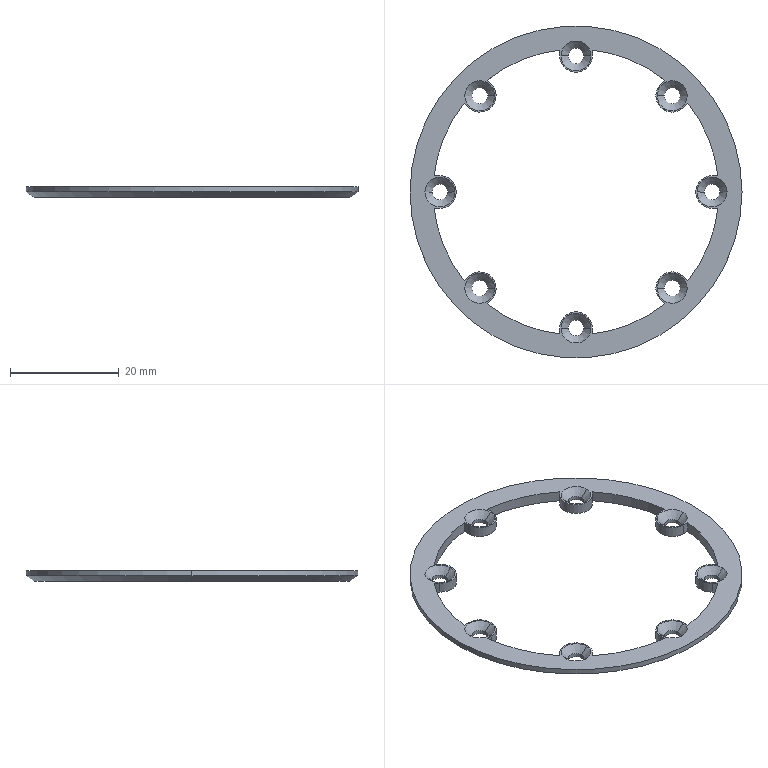Part | SolidWorks | features Chamfer 1, CirPattern 1, Extrusion 1, HoleWzd 1, ICE 1 | 1 solid | 73 faces | box 61 x 61 x 2 mm | volume 1529 mm3 | cylinder 37 | cone 18 | plane 18 | commonest cylinder face diameters 2.9 x16 6 x11 52.5 x8 61 x2